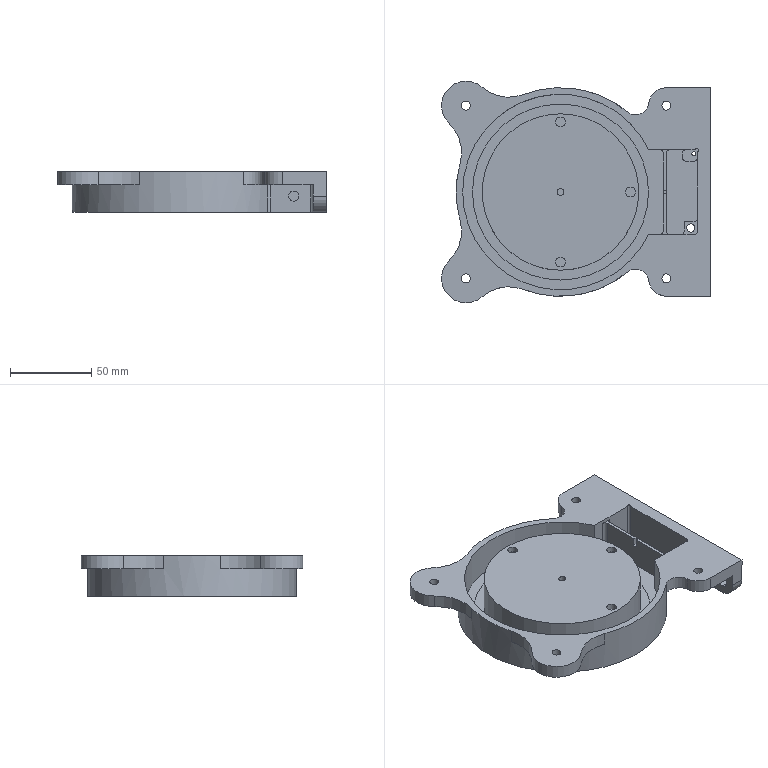NC program | NX | posted with a generic post | part box 165 x 136 x 25 mm
Lines 71 to 1171 of 16615:
(ADAPTIVE_MILLING , TOOL : D10)
N122 T10 M6
N124 G54
N126 G17 G0 G90 X95.139 Y-52.783 S9500 M3
N128 G43 Z30. H10
N130 Z-22.
N132 G94 G1 Z-25. F1000.
N134 X93.885 Y-52.222 F2500.
N136 G3 X92.53 Y-52.783 R1.011
N138 X92.255 Y-53.961 R4.871
N140 X92.058 Y-56.953 R29.061
N142 X92.005 Y-64.578 R349.415
N144 G1 X92.004 Y-66.453
N146 Y-70.016
N148 Y-70.766
N150 Y-70.828
N152 X92.003 Y-70.891
N154 X92.002 Y-70.953
N156 X92. Y-71.015
N158 G2 X90.865 Y-74.007 R5.312
N160 X88.246 Y-76.088 R7.29
N162 X85.091 Y-77.059 R11.809
N164 X81.36 Y-77.407 R28.55
N166 X75.735 Y-77.488 R162.167
N168 G1 X74.923 Y-77.49
N170 X73.985 Y-77.492
N172 X72.673 Y-77.493
N174 X70.798 Y-77.494
N176 X67.36 Y-77.495
N178 X25.735 Y-77.494
N180 X-85.327
N182 X-85.39 Y-77.493
N184 X-85.452 Y-77.492
N186 X-85.515 Y-77.49
N188 G2 X-88.556 Y-76.317 R5.341
N190 X-90.614 Y-73.68 R7.344
N192 X-91.569 Y-70.52 R11.916
N194 X-91.912 Y-66.725 R29.474
N196 X-91.99 Y-60.351 R197.421
N198 G1 X-91.992 Y-59.413
N200 X-91.993 Y-58.101
N202 X-91.994 Y-56.163
N204 X-91.995 Y-52.663
N206 Y6.837
N208 Y70.837
N210 G2 X-90.961 Y73.863 R5.24
N212 X-88.45 Y75.977 R7.1
N214 X-85.317 Y77.014 R11.258
N216 X-81.839 Y77.383 R25.481
N218 X-76.09 Y77.485 R135.933
N220 G1 X-75.34 Y77.488
N222 X-74.465 Y77.489
N224 X-73.403 Y77.491
N226 X-71.903 Y77.492
N228 X-69.528 Y77.493
N230 X-64.09
N232 X-3.653
N234 X-3.403 Y77.494
N236 X85.347
N238 X85.41 Y77.493
N240 X85.472 Y77.492
N242 X85.535 Y77.489
N244 G2 X88.571 Y76.303 R5.343
N246 X90.594 Y73.716 R7.325
N248 X91.56 Y70.559 R11.808
N250 X91.904 Y66.89 R28.115
N252 X91.987 Y61.079 R165.071
N254 G1 X91.989 Y60.266
N256 X91.991 Y59.204
N258 X91.992 Y57.766
N260 X91.993 Y55.641
N262 Y51.266
N264 Y-50.109
N266 X91.992 Y-50.234
N268 X91.991 Y-50.296
N270 X91.99 Y-50.359
N272 G2 X91.814 Y-52.977 R46.721
N274 G3 X91.533 Y-59.97 R91.09
N276 X91.508 Y-68.782 R942.218
N278 G2 X89.291 Y-73.791 R7.073
N280 X86.183 Y-75.732 R9.353
N282 X82.611 Y-76.611 R15.534
N284 X78.374 Y-76.917 R40.348
N286 X70.625 Y-76.987 R304.917
N288 G1 X69.125 Y-76.988
N290 X66.937 Y-76.989
N292 X62.687
N294 X-83.125 Y-76.988
N296 X-83.188
N298 X-83.25
N300 G2 X-88.27 Y-74.797 R7.053
N302 X-90.288 Y-71.521 R9.391
N304 X-91.132 Y-67.94 R16.006
N306 X-91.425 Y-63.514 R44.133
N308 X-91.487 Y-55.952 R338.286
N310 G1 X-91.488 Y-54.452
N312 X-91.489 Y-52.265
N314 Y-47.952
N316 Y-10.577
N318 X-91.491 Y-10.265
N320 Y-9.702
N322 X-91.492 Y-9.39
N324 X-91.491 Y-7.202
N326 X-91.492 Y-6.89
N328 X-91.491 Y-4.702
N330 X-91.492 Y-4.39
N332 X-91.491 Y-2.202
N334 X-91.492 Y-1.89
N336 X-91.491 Y0.298
N338 X-91.492 Y0.61
N340 X-91.491 Y2.798
N342 X-91.492 Y3.11
N344 X-91.491 Y5.298
N346 X-91.492 Y5.61
N348 X-91.491 Y7.798
N350 X-91.492 Y8.11
N352 X-91.491 Y10.298
N354 X-91.492 Y10.61
N356 X-91.491 Y12.798
N358 X-91.492 Y13.11
N360 X-91.491 Y15.298
N362 X-91.492 Y15.61
N364 X-91.491 Y17.798
N366 X-91.492 Y18.11
N368 X-91.491 Y20.298
N370 X-91.492 Y20.61
N372 X-91.491 Y22.798
N374 X-91.492 Y23.11
N376 X-91.491 Y25.298
N378 X-91.492 Y25.61
N380 X-91.491 Y27.798
N382 X-91.492 Y28.11
N384 X-91.491 Y30.298
N386 X-91.492 Y30.61
N388 X-91.491 Y32.798
N390 X-91.492 Y33.11
N392 X-91.491 Y35.298
N394 X-91.492 Y35.61
N396 X-91.491 Y37.798
N398 X-91.492 Y38.11
N400 X-91.491 Y40.298
N402 X-91.492 Y40.61
N404 X-91.491 Y42.798
N406 X-91.492 Y43.11
N408 X-91.491 Y45.298
N410 X-91.492 Y45.61
N412 X-91.491 Y47.798
N414 X-91.492 Y48.11
N416 X-91.491 Y50.298
N418 X-91.492 Y50.61
N420 X-91.491 Y52.798
N422 X-91.492 Y53.11
N424 X-91.491 Y55.298
N426 X-91.492 Y55.61
N428 X-91.491 Y57.798
N430 X-91.492 Y58.11
N432 X-91.491 Y60.298
N434 X-91.492 Y60.61
N436 X-91.491 Y62.798
N438 X-91.492 Y63.11
N440 X-91.491 Y65.298
N442 G2 X-91.484 Y68.985 R228.266
N444 X-89.309 Y73.758 R7.041
N446 X-86.094 Y75.758 R9.386
N448 X-82.455 Y76.628 R15.836
N450 X-78.405 Y76.914 R40.706
N452 X-70.968 Y76.984 R288.617
N454 G1 X-69.655 Y76.986
N456 X-67.843 Y76.987
N458 X-64.843
N460 X-55.405 Y76.988
N462 X-5.843
N464 X-5.718
N466 X-5.093 Y76.989
N468 X83.157
N470 X83.22 Y76.988
N472 X83.282 Y76.987
N474 X83.407 Y76.984
N476 G2 X88.291 Y74.772 R7.043
N478 X90.298 Y71.49 R9.465
N480 X91.136 Y67.907 R16.208
N482 X91.429 Y63.356 R44.995
N484 X91.487 Y54.419 R442.168
N486 G1 Y52.106
N488 X91.488 Y47.356
N490 Y-48.331
N492 X91.486 Y-48.581
N494 X91.485 Y-48.769
N496 X91.483 Y-48.956
N498 G2 X91.288 Y-53.014 R91.927
N500 G3 X91.035 Y-61.509 R150.124
N502 G1 X91.032 Y-62.071
N504 X91.028 Y-62.696
N506 X91.025 Y-63.384
N508 X91.023 Y-64.196
N510 X91.02 Y-65.134
N512 X91.018 Y-66.259
N514 Y-66.446
N516 X91.016 Y-66.696
N518 X91.015 Y-66.821
N520 Y-66.884
N522 X91.012 Y-67.009
N524 X91.011 Y-67.071
N526 G2 X90.235 Y-70.584 R8.586
N528 X87.223 Y-74.019 R8.505
N530 X83.634 Y-75.595 R12.014
N532 X79.629 Y-76.246 R22.581
N534 X74.759 Y-76.445 R71.997
N536 X63.009 Y-76.484 R974.246
N538 G1 X56.322
N540 X-7.491 Y-76.483
N542 X-7.803 Y-76.485
N544 X-8.366
N546 X-8.678 Y-76.486
N548 X-10.866 Y-76.485
N550 X-11.178 Y-76.486
N552 X-13.366 Y-76.485
N554 X-13.678 Y-76.486
N556 X-15.866 Y-76.485
N558 X-16.178 Y-76.486
N560 X-18.366 Y-76.485
N562 X-18.678 Y-76.486
N564 X-20.866 Y-76.485
N566 X-21.178 Y-76.486
N568 X-23.366 Y-76.485
N570 X-23.678 Y-76.486
N572 X-25.866 Y-76.485
N574 X-26.178 Y-76.486
N576 X-28.366 Y-76.485
N578 X-28.678 Y-76.486
N580 X-30.866 Y-76.485
N582 X-31.178 Y-76.486
N584 X-33.366 Y-76.484
N586 X-33.678 Y-76.486
N588 X-35.866 Y-76.484
N590 X-36.178 Y-76.486
N592 X-38.366 Y-76.484
N594 X-38.678 Y-76.486
N596 X-40.866 Y-76.484
N598 X-41.178 Y-76.486
N600 X-43.366 Y-76.484
N602 X-43.678 Y-76.486
N604 X-45.866 Y-76.484
N606 X-46.178 Y-76.486
N608 X-48.366 Y-76.484
N610 X-48.678 Y-76.486
N612 X-50.866 Y-76.484
N614 X-51.178 Y-76.486
N616 X-53.366 Y-76.484
N618 X-53.678 Y-76.486
N620 X-55.866 Y-76.484
N622 X-56.178 Y-76.486
N624 X-58.366 Y-76.484
N626 X-58.678 Y-76.486
N628 X-60.866 Y-76.484
N630 X-61.178 Y-76.486
N632 X-63.366 Y-76.484
N634 X-63.678 Y-76.485
N636 X-65.866 Y-76.484
N638 X-66.178 Y-76.485
N640 X-68.366 Y-76.484
N642 X-68.678 Y-76.485
N644 X-70.866 Y-76.484
N646 X-71.178 Y-76.485
N648 X-73.366 Y-76.484
N650 X-73.678 Y-76.485
N652 X-75.866 Y-76.484
N654 X-76.178 Y-76.485
N656 X-78.366 Y-76.484
N658 G2 X-81.803 Y-76.473 R148.791
N660 X-86.051 Y-75.172 R8.179
N662 X-88.905 Y-72.078 R8.912
N664 X-90.257 Y-68.462 R13.076
N666 X-90.794 Y-64.439 R26.277
N668 X-90.962 Y-58.692 R100.92
N670 X-90.984 Y-49.317 R958.544
N672 G1 Y-44.505
N674 Y-12.755
N676 X-90.985 Y-12.505
N678 X-90.986 Y-11.63
N680 X-90.987 Y-11.317
N682 Y-10.692
N684 X-90.986 Y-9.38
N686 X-90.987 Y-9.13
N688 Y-7.942
N690 Y-7.255
N692 X-90.988 Y-6.942
N694 Y-6.567
N696 X-90.989 Y-6.255
N698 Y-5.942
N700 X-90.99 Y-5.442
N702 X-90.989 Y-4.317
N704 X-90.99 Y-4.005
N706 X-90.989 Y-3.192
N708 X-90.99 Y-2.817
N710 X-90.989 Y-1.755
N712 Y-1.505
N714 X-90.988 Y-0.317
N716 X-90.989 Y-0.005
N718 X-90.988 Y0.745
N720 X-90.989 Y0.933
N722 Y1.558
N724 X-90.99 Y1.87
N726 X-90.988 Y3.183
N728 X-90.989 Y3.433
N730 X-90.988 Y4.62
N732 X-90.989 Y4.933
N734 X-90.988 Y5.808
N736 X-90.989 Y5.995
N738 Y6.558
N740 X-90.988 Y6.745
N742 X-90.989 Y7.058
N744 X-90.988 Y8.245
N746 X-90.989 Y8.495
N748 X-90.988 Y9.683
N750 Y9.87
N752 X-90.989 Y10.183
N754 X-90.988 Y10.808
N756 X-90.989 Y10.933
N758 X-90.988 Y11.62
N760 Y11.745
N762 X-90.989 Y12.058
N764 X-90.988 Y13.245
N766 X-90.989 Y13.495
N768 X-90.988 Y14.683
N770 Y14.808
N772 X-90.989 Y15.12
N774 X-90.988 Y15.808
N776 X-90.989 Y15.995
N778 Y16.62
N780 X-90.99 Y16.933
N782 X-90.988 Y18.183
N784 X-90.989 Y18.433
N786 X-90.988 Y19.558
N788 X-90.989 Y19.87
N790 X-90.988 Y20.745
N792 X-90.989 Y20.933
N794 Y21.37
N796 X-90.988 Y21.745
N798 X-90.989 Y22.058
N800 X-90.988 Y23.245
N802 X-90.989 Y23.433
N804 X-90.988 Y24.058
N806 X-90.989 Y24.37
N808 X-90.988 Y25.745
N810 X-90.989 Y25.995
N812 X-90.988 Y27.183
N814 Y27.308
N816 X-90.989 Y27.62
N818 X-90.988 Y28.308
N820 X-90.989 Y28.433
N822 X-90.988 Y29.058
N824 Y29.433
N826 X-90.989 Y29.745
N828 X-90.988 Y30.808
N830 X-90.989 Y30.995
N832 X-90.988 Y31.558
N834 Y31.745
N836 X-90.989 Y32.058
N838 X-90.988 Y33.245
N840 X-90.989 Y33.433
N842 Y33.87
N844 X-90.988 Y34.12
N846 X-90.989 Y34.433
N848 X-90.988 Y35.745
N850 X-90.989 Y35.933
N852 X-90.988 Y36.558
N854 X-90.989 Y36.87
N856 X-90.988 Y38.245
N858 X-90.989 Y38.433
N860 X-90.988 Y38.87
N862 Y39.12
N864 X-90.989 Y39.433
N866 X-90.988 Y40.745
N868 X-90.989 Y40.933
N870 Y41.37
N872 X-90.988 Y41.745
N874 X-90.989 Y42.058
N876 X-90.988 Y43.245
N878 X-90.989 Y43.433
N880 X-90.988 Y44.058
N882 Y44.12
N884 X-90.989 Y44.433
N886 X-90.988 Y45.683
N888 X-90.989 Y45.933
N890 X-90.988 Y47.058
N892 Y47.308
N894 X-90.989 Y47.62
N896 X-90.988 Y48.308
N898 X-90.989 Y48.433
N900 X-90.988 Y49.12
N902 Y49.37
N904 X-90.989 Y49.683
N906 X-90.988 Y50.745
N908 X-90.99 Y51.245
N910 Y51.37
N912 X-90.991 Y51.87
N914 X-90.989 Y52.87
N916 X-90.991 Y53.683
N918 X-90.989 Y54.745
N920 X-90.99 Y55.12
N922 X-90.989 Y55.745
N924 X-90.99 Y55.995
N926 X-90.989 Y56.933
N928 X-90.99 Y57.308
N930 X-90.989 Y58.245
N932 X-90.99 Y58.495
N934 X-90.988 Y59.62
N936 X-90.99 Y59.995
N938 X-90.989 Y60.808
N940 Y60.995
N942 Y61.433
N944 Y61.808
N946 X-90.99 Y62.183
N948 X-90.989 Y62.433
N950 X-90.99 Y62.808
N952 Y63.245
N954 Y63.433
N956 G2 X-90.979 Y67.245 R266.112
N958 X-89.87 Y71.236 R8.244
N960 X-86.737 Y74.312 R8.787
N962 X-83.14 Y75.714 R12.825
N964 X-79.185 Y76.277 R25.023
N966 X-74.001 Y76.453 R86.031
N968 X-63.251 Y76.482 R987.32
N970 G1 X-57.126
N972 X-26.314
N974 X-26.001 Y76.484
N976 X-25.439 Y76.483
N978 X-25.126 Y76.485
N980 X-22.939 Y76.483
N982 X-22.626 Y76.485
N984 X-20.439 Y76.483
N986 X-20.126 Y76.485
N988 X-17.939 Y76.483
N990 X-17.626 Y76.485
N992 X-15.439 Y76.483
N994 X-15.126 Y76.485
N996 X-12.939 Y76.483
N998 X-12.626 Y76.485
N1000 X-10.439 Y76.483
N1002 X-10.126 Y76.485
N1004 X-8.001 Y76.483
N1006 X-7.814 Y76.484
N1008 X-6.501
N1010 X-6.314
N1012 X-6.001 Y76.485
N1014 X-3.376 Y76.484
N1016 X-3.064 Y76.485
N1018 X-0.314 Y76.484
N1020 X-0.001 Y76.486
N1022 X2.749 Y76.484
N1024 X3.061 Y76.486
N1026 X5.874 Y76.484
N1028 X6.186 Y76.486
N1030 X8.936 Y76.484
N1032 X9.249 Y76.486
N1034 X12.061 Y76.484
N1036 X12.374 Y76.486
N1038 X15.124 Y76.484
N1040 X15.436 Y76.486
N1042 X18.249 Y76.484
N1044 X18.561 Y76.486
N1046 X21.311 Y76.484
N1048 X21.624 Y76.486
N1050 X24.436 Y76.484
N1052 X24.749 Y76.486
N1054 X27.499 Y76.484
N1056 X27.811 Y76.486
N1058 X30.624 Y76.484
N1060 X30.936 Y76.486
N1062 X33.749 Y76.484
N1064 X34.061 Y76.486
N1066 X36.811 Y76.484
N1068 X37.124 Y76.486
N1070 X39.936 Y76.484
N1072 X40.249 Y76.486
N1074 X42.999 Y76.484
N1076 X43.311 Y76.486
N1078 X46.124 Y76.484
N1080 X46.436 Y76.486
N1082 X49.186 Y76.484
N1084 X49.499 Y76.486
N1086 X52.311 Y76.484
N1088 X52.624 Y76.486
N1090 X55.374 Y76.484
N1092 X55.686 Y76.486
N1094 X58.499 Y76.484
N1096 X58.811 Y76.486
N1098 X61.561 Y76.484
N1100 X61.874 Y76.486
N1102 X64.686 Y76.484
N1104 X64.999 Y76.486
N1106 X67.749 Y76.484
N1108 X68.061 Y76.486
N1110 X70.874 Y76.484
N1112 X71.186 Y76.486
N1114 X73.936 Y76.484
N1116 X74.249 Y76.486
N1118 X77.061 Y76.484
N1120 X77.374 Y76.486
N1122 X80.124 Y76.484
N1124 X80.436 Y76.486
N1126 X81.186 Y76.485
N1128 X81.374 Y76.484
N1130 X81.436
N1132 X81.561 Y76.481
N1134 G2 X85.076 Y75.714 R8.483
N1136 X88.617 Y72.55 R8.518
N1138 X90.125 Y68.999 R12.224
N1140 X90.756 Y64.991 R23.353
N1142 X90.95 Y59.808 R79.617
N1144 X90.982 Y50.433 R858.768
N1146 G1 Y46.933
N1148 X90.983 Y30.495
N1150 X90.982 Y-47.005
N1152 X90.981 Y-47.255
N1154 X90.978 Y-47.567
N1156 G2 X90.795 Y-52.626 R117.036
N1158 G3 X90.538 Y-62.934 R211.978
N1160 G2 X90.5 Y-65.996 R87.112
N1162 X89.684 Y-69.569 R9.654
N1164 X86.365 Y-73.385 R9.11
N1166 X82.662 Y-75.014 R12.786
N1168 X78.6 Y-75.701 R23.382
N1170 X73.481 Y-75.932 R70.527
N1172 X62.356 Y-75.978 R790.426
N1174 G1 X58.356
N1176 X21.731
N1178 X-5.331
N1180 X-5.644 Y-75.98
N1182 X-6.206
N1184 X-6.581 Y-75.981
N1186 X-7.581
N1188 X-8.269
N1190 X-8.581 Y-75.982
N1192 X-9.019
N1194 X-9.331 Y-75.983
N1196 X-9.769 Y-75.982
N1198 X-10.206 Y-75.984
N1200 X-10.456 Y-75.983
N1202 X-10.831 Y-75.984
N1204 X-11.393 Y-75.983
N1206 X-11.581 Y-75.984
N1208 X-12.831 Y-75.983
N1210 X-13.206 Y-75.984
N1212 X-13.893 Y-75.983
N1214 X-14.081
N1216 X-14.706
N1218 X-14.831
N1220 X-15.518
N1222 X-15.893 Y-75.984
N1224 X-16.393 Y-75.983
N1226 X-16.581 Y-75.984
N1228 X-17.206 Y-75.983
N1230 X-17.331
N1232 X-18.831 Y-75.982
N1234 X-19.018 Y-75.983
N1236 X-19.581 Y-75.982
N1238 X-19.768
N1240 X-19.893 Y-75.983
N1242 X-20.893 Y-75.982
N1244 X-21.143
N1246 X-21.518 Y-75.983
N1248 X-22.331 Y-75.982
N1250 X-22.706 Y-75.984
N1252 X-23.018 Y-75.983
N1254 X-23.643 Y-75.985
N1256 X-23.956 Y-75.984
N1258 X-24.581 Y-75.986
N1260 X-24.706 Y-75.985
N1262 X-25.456 Y-75.987
N1264 X-26.081 Y-75.985
N1266 X-26.643 Y-75.986
N1268 X-26.768
N1270 X-27.456 Y-75.987
N1272 X-28.081 Y-75.985
N1274 X-29.268 Y-75.987
N1276 X-29.893 Y-75.986
N1278 X-30.518 Y-75.987
N1280 X-31.143 Y-75.985
N1282 X-31.643 Y-75.986
N1284 X-31.768
N1286 X-32.456 Y-75.987
N1288 X-33.081 Y-75.985
N1290 X-34.268 Y-75.987
N1292 X-34.893 Y-75.986
N1294 X-35.518 Y-75.987
N1296 X-36.143 Y-75.985
N1298 X-36.706 Y-75.986
N1300 X-36.831
N1302 X-37.706 Y-75.987
N1304 X-37.831
N1306 X-39.268 Y-75.988
N1308 X-39.768 Y-75.987
N1310 X-40.456
N1312 X-40.956 Y-75.986
N1314 X-41.581 Y-75.987
N1316 X-41.706 Y-75.986
N1318 X-43.018 Y-75.988
N1320 X-44.331 Y-75.989
N1322 X-45.643
N1324 X-46.956 Y-75.988
N1326 X-48.268 Y-75.986
N1328 X-49.518 Y-75.984
N1330 X-50.018 Y-75.985
N1332 X-50.143
N1334 X-50.956 Y-75.986
N1336 X-51.081
N1338 X-51.768 Y-75.987
N1340 X-51.893
N1342 X-52.018
N1344 X-53.331 Y-75.988
N1346 X-54.643 Y-75.989
N1348 X-55.956 Y-75.988
N1350 X-57.268
N1352 X-58.581 Y-75.986
N1354 X-59.706 Y-75.984
N1356 X-60.143 Y-75.985
N1358 X-61.018 Y-75.983
N1360 X-61.956 Y-75.986
N1362 X-62.081 Y-75.985
N1364 X-62.893 Y-75.987
N1366 X-63.018 Y-75.986
N1368 X-64.581 Y-75.988
N1370 X-65.081 Y-75.986
N1372 X-65.768 Y-75.987
N1374 X-66.206 Y-75.986
N1376 X-66.768 Y-75.987
N1378 X-66.893 Y-75.986
N1380 X-67.768 Y-75.987
N1382 X-67.893
N1384 X-69.331 Y-75.988
N1386 X-69.456
N1388 X-69.956 Y-75.987
N1390 X-70.768
N1392 X-71.206 Y-75.986
N1394 X-71.831 Y-75.987
N1396 X-72.456 Y-75.985
N1398 X-73.081 Y-75.986
N1400 X-73.706 Y-75.985
N1402 X-74.268 Y-75.986
N1404 G2 X-80.143 Y-75.976 R612.966
N1406 X-83.277 Y-75.467 R10.413
N1408 X-87.615 Y-72.23 R8.912
N1410 X-89.383 Y-68.593 R12.154
N1412 X-90.147 Y-64.609 R21.448
N1414 X-90.418 Y-59.681 R58.799
N1416 X-90.477 Y-49.744 R542.864
N1418 G1 X-90.478 Y-47.369
N1420 X-90.479 Y-42.806
N1422 Y-14.931
N1424 X-90.48 Y-14.619
N1426 Y-13.744
N1428 X-90.482 Y-13.494
N1430 Y-12.431
N1432 Y-11.556
N1434 X-90.483 Y-11.244
N1436 Y-10.181
N1438 Y-9.431
N1440 X-90.484 Y-9.181
N1442 Y-8.494
N1444 Y-8.369
N1446 X-90.485 Y-7.806
N1448 Y-7.619
N1450 Y-6.994
N1452 Y-6.494
N1454 X-90.486 Y-6.181
N1456 Y-5.244
N1458 Y-5.056
N1460 Y-4.619
N1462 Y-3.931
N1464 X-90.487 Y-3.681
N1466 X-90.486 Y-2.556
N1468 Y-2.431
N1470 Y-2.181
N1472 Y-1.244
N1474 X-90.487 Y-0.869
N1476 Y-0.619
N1478 X-90.488 Y0.006
N1480 Y0.444
N1482 X-90.489 Y0.881
N1484 X-90.488 Y1.256
N1486 X-90.489 Y1.756
N1488 X-90.487 Y2.569
N1490 X-90.488 Y2.881
N1492 X-90.487 Y3.694
N1494 X-90.488 Y3.944
N1496 X-90.487 Y4.694
N1498 Y4.944
N1500 X-90.486 Y6.006
N1502 X-90.487 Y6.319
N1504 X-90.486 Y7.069
N1506 X-90.487 Y7.381
N1508 X-90.486 Y7.944
N1510 X-90.487 Y8.069
N1512 X-90.486 Y8.756
N1514 X-90.487 Y8.881
N1516 X-90.486 Y9.756
N1518 Y9.881
N1520 Y10.569
N1522 X-90.485 Y11.069
N1524 X-90.486 Y11.381
N1526 X-90.485 Y12.381
N1528 X-90.487 Y13.006
N1530 Y13.194
N1532 X-90.489 Y14.256
N1534 X-90.491 Y15.381
N1536 X-90.492 Y16.506
N1538 Y17.631
N1540 X-90.491 Y18.756
N1542 X-90.49 Y19.881
N1544 X-90.488 Y20.819
N1546 X-90.489 Y21.569
N1548 X-90.488 Y22.006
N1550 X-90.489 Y22.256
N1552 X-90.487 Y23.194
N1554 X-90.489 Y23.944
N1556 X-90.487 Y24.819
N1558 X-90.489 Y25.631
N1560 Y25.756
N1562 X-90.49 Y26.694
N1564 X-90.489 Y27.319
N1566 X-90.49 Y27.756
N1568 X-90.489 Y28.131
N1570 X-90.49 Y29.194
N1572 X-90.489 Y29.694
N1574 X-90.49 Y30.006
N1576 X-90.488 Y30.631
N1578 X-90.49 Y31.381
N1580 X-90.488 Y32.006
N1582 X-90.489 Y32.381
N1584 X-90.488 Y33.006
N1586 X-90.489 Y33.381
N1588 X-90.488 Y33.756
N1590 X-90.489 Y34.319
N1592 X-90.488 Y34.631
N1594 X-90.49 Y35.131
N1596 X-90.487 Y36.131
N1598 X-90.488 Y36.381
N1600 X-90.487 Y37.006
N1602 X-90.488 Y37.319
N1604 X-90.487 Y38.194
N1606 X-90.488 Y38.569
N1608 X-90.487 Y39.006
N1610 X-90.488 Y39.381
N1612 X-90.487 Y39.756
N1614 X-90.489 Y40.256
N1616 X-90.488 Y40.444
N1618 X-90.489 Y40.881
N1620 X-90.488 Y41.256
N1622 X-90.489 Y41.756
N1624 X-90.488 Y42.131
N1626 X-90.49 Y42.694
N1628 X-90.488 Y43.569
N1630 Y43.881
N1632 X-90.487 Y44.569
N1634 X-90.488 Y44.944
N1636 X-90.487 Y45.319
N1638 X-90.489 Y45.819
N1640 X-90.487 Y46.444
N1642 X-90.488 Y46.881
N1644 Y47.381
N1646 Y47.569
N1648 X-90.487 Y48.131
N1650 X-90.488 Y48.506
N1652 Y48.819
N1654 X-90.489 Y49.194
N1656 X-90.488 Y49.631
N1658 X-90.489 Y49.944
N1660 X-90.488 Y50.694
N1662 X-90.489 Y51.194
N1664 X-90.487 Y52.694
N1666 X-90.488 Y52.881
N1668 X-90.487 Y53.506
N1670 Y53.569
N1672 X-90.488 Y53.881
N1674 X-90.487 Y54.756
N1676 X-90.488 Y55.131
N1678 X-90.487 Y56.069
N1680 X-90.488 Y56.381
N1682 X-90.487 Y57.319
N1684 X-90.489 Y58.069
N1686 X-90.488 Y58.319
N1688 X-90.49 Y58.944
N1690 X-90.489 Y59.069
N1692 X-90.49 Y59.569
N1694 X-90.489 Y59.881
N1696 X-90.491 Y60.819
N1698 Y60.944
N1700 X-90.492 Y61.881
N1702 X-90.49 Y62.444
N1704 G2 X-90.475 Y65.818 R135.493
N1706 X-89.824 Y69.176 R9.958
N1708 X-86.589 Y73.216 R8.972
N1710 X-82.927 Y74.932 R12.352
N1712 X-78.937 Y75.666 R22.255
N1714 X-73.82 Y75.924 R63.881
N1716 X-64.257 Y75.975 R594.582
N1718 G1 X-61.82 Y75.976
N1720 X-57.195 Y75.977
N1722 X-28.507
N1724 X-28.382
N1726 X-27.757 Y75.978
N1728 X-27.632
N1730 X-27.445 Y75.979
N1732 X-26.507
N1734 X-25.132
N1736 X-25.007
N1738 X-24.507 Y75.98
N1740 X-22.632 Y75.979
N1742 X-22.507
N1744 X-22.007 Y75.98
N1746 X-20.132 Y75.979
N1748 X-20.007 Y75.98
N1750 X-19.507
N1752 X-17.632 Y75.979
N1754 X-17.507 Y75.98
N1756 X-17.007
N1758 X-15.132 Y75.979
N1760 X-15.007 Y75.98
N1762 X-14.507
N1764 X-12.507 Y75.979
N1766 X-12.32 Y75.98
N1768 X-11.695
N1770 X-10.445 Y75.979
N1772 X-9.945 Y75.981
N1774 X-8.382 Y75.98
N1776 X-8.195 Y75.981
N1778 X-7.632
N1780 X-6.882
N1782 X-6.57 Y75.982
N1784 X-6.257
N1786 X-5.757 Y75.983
N1788 X-5.382
N1790 X-4.882 Y75.984
N1792 X-3.632 Y75.982
N1794 X-3.257 Y75.984
N1796 X-2.382 Y75.982
N1798 X-2.132 Y75.983
N1800 X-1.132 Y75.982
N1802 X-0.82 Y75.983
N1804 X0.555 Y75.982
N1806 X0.868 Y75.983
N1808 X1.68 Y75.982
N1810 X1.993 Y75.983
N1812 X3.618 Y75.981
N1814 X4.305 Y75.984
N1816 X6.055 Y75.982
N1818 X6.368 Y75.983
N1820 X6.93 Y75.982
N1822 X7.118 Y75.983
N1824 X7.743 Y75.982
N1826 X8.118 Y75.984
N1828 X9.868 Y75.982
N1830 X10.18 Y75.983
N1832 X10.993 Y75.982
N1834 X11.305 Y75.983
N1836 X12.93 Y75.981
N1838 X13.243 Y75.982
N1840 X14.18
N1842 X14.493 Y75.983
N1844 X16.118 Y75.981
N1846 X16.368 Y75.982
N1848 X17.493
N1850 X17.743 Y75.981
N1852 X18.055 Y75.983
N1854 X19.305 Y75.981
N1856 X19.493 Y75.982
N1858 X20.055
N1860 X20.305
N1862 X20.618 Y75.983
N1864 X22.368 Y75.981
N1866 X22.618 Y75.982
N1868 X23.805
N1870 X24.055 Y75.981
N1872 X24.368 Y75.982
N1874 X25.493
N1876 X25.68
N1878 X26.243
N1880 X26.618
N1882 X26.93 Y75.983
N1884 X28.555 Y75.981
N1886 X28.805 Y75.982
N1888 X29.993
N1890 X30.18 Y75.981
N1892 X30.493 Y75.983
N1894 X31.68 Y75.981
N1896 X32.18 Y75.983
N1898 X34.618 Y75.981
N1900 X34.93 Y75.982
N1902 X35.93
N1904 X36.243 Y75.983
N1906 X37.868 Y75.981
N1908 X38.118 Y75.982
N1910 X39.305
N1912 X39.493
N1914 X39.805 Y75.983
N1916 X40.93 Y75.982
N1918 X41.118
N1920 X41.68
N1922 X41.868
N1924 X42.18 Y75.983
N1926 X43.993 Y75.981
N1928 X44.18 Y75.982
N1930 X44.743
N1932 X45.055 Y75.983
N1934 X46.993 Y75.981
N1936 X47.305 Y75.982
N1938 X48.305
N1940 X48.618 Y75.983
N1942 X50.243 Y75.981
N1944 X50.43 Y75.982
N1946 X50.868
N1948 X51.243
N1950 X51.555 Y75.983
N1952 X53.305 Y75.981
N1954 X53.493 Y75.982
N1956 X53.93
N1958 X54.243
N1960 X54.555 Y75.983
N1962 X56.43 Y75.981
N1964 X56.618 Y75.982
N1966 X57.055
N1968 X57.43
N1970 X57.743 Y75.983
N1972 X59.493 Y75.981
N1974 X59.618 Y75.982
N1976 X60.243
N1978 X60.493 Y75.981
N1980 X60.805 Y75.983
N1982 X62.68 Y75.981
N1984 X62.868 Y75.982
N1986 X63.43
N1988 X63.93 Y75.981
N1990 X64.243 Y75.983
N1992 X65.743 Y75.981
N1994 X65.93 Y75.982
N1996 X66.493
N1998 X66.93
N2000 X67.243 Y75.983
N2002 X68.805 Y75.981
N2004 X68.993 Y75.982
N2006 X69.618
N2008 X69.93 Y75.983
N2010 X71.805 Y75.981
N2012 X72.117 Y75.982
N2014 X73.242
N2016 X73.555 Y75.983
N2018 X74.992 Y75.981
N2020 X75.18 Y75.982
N2022 X75.742
N2024 X76.055 Y75.983
N2026 X77.617 Y75.981
N2028 G2 X80.555 Y75.959 R68.776
N2030 X84.237 Y75.075 R9.482
N2032 X87.92 Y71.786 R9.144
N2034 X89.531 Y68.075 R12.828
N2036 X90.218 Y63.887 R23.879
N2038 X90.44 Y58.393 R80.072
N2040 X90.476 Y48.518 R864.782
N2042 G1 X90.477 Y45.205
N2044 Y34.83
N2046 Y-45.982
N2048 X90.476 Y-46.17
N2050 X90.474 Y-46.42
N2052 G2 X90.291 Y-52.479 R153.217
N2054 G3 X90.045 Y-63.038 R269.347
N2056 G2 X89.943 Y-65.535 R26.924
N2058 X88.544 Y-69.77 R9.815
N2060 X85.046 Y-73.097 R10.027
N2062 X81.156 Y-74.604 R14.293
N2064 X76.706 Y-75.242 R27.866
N2066 X70.836 Y-75.441 R96.727
N2068 X60.898 Y-75.472 R914.91
N2070 G1 X57.398 Y-75.473
N2072 X45.648
N2074 X-3.102
N2076 X-3.789 Y-75.476
N2078 X-3.914
N2080 X-4.477 Y-75.478
N2082 X-4.727
N2084 X-4.977 Y-75.479
N2086 X-5.352 Y-75.478
N2088 X-5.727 Y-75.479
N2090 X-6.164
N2092 X-6.414 Y-75.48
N2094 X-6.977 Y-75.479
N2096 X-7.414 Y-75.481
N2098 X-7.602 Y-75.48
N2100 X-8.102 Y-75.482
N2102 X-8.289
N2104 X-8.789 Y-75.483
N2106 X-10.102 Y-75.481
N2108 X-10.414 Y-75.482
N2110 X-10.914 Y-75.481
N2112 X-11.289 Y-75.482
N2114 X-12.227 Y-75.481
N2116 X-12.664 Y-75.482
N2118 X-13.539 Y-75.481
N2120 X-13.977 Y-75.482
N2122 X-14.727 Y-75.481
N2124 X-15.164 Y-75.483
N2126 X-16.789 Y-75.48
N2128 X-17.227 Y-75.481
N2130 X-18.039 Y-75.48
N2132 X-18.352 Y-75.481
N2134 X-19.102 Y-75.48
N2136 X-19.352 Y-75.481
N2138 X-20.289 Y-75.48
N2140 X-20.539 Y-75.481
N2142 X-21.164 Y-75.48
N2144 X-21.289 Y-75.481
N2146 X-22.164
N2148 X-22.539 Y-75.482
N2150 X-23.102
N2152 X-23.352 Y-75.483
N2154 X-23.977 Y-75.482
N2156 X-24.102
N2158 X-24.289 Y-75.483
N2160 X-24.852
N2162 X-25.289 Y-75.484
N2164 X-25.977 Y-75.483
N2166 X-26.914 Y-75.486
N2168 X-28.102 Y-75.484
N2170 X-28.477 Y-75.485
N2172 X-29.039 Y-75.484
N2174 X-29.227 Y-75.485
N2176 X-29.664 Y-75.484
N2178 X-30.352 Y-75.486
N2180 X-30.977 Y-75.485
N2182 X-32.227 Y-75.487
N2184 X-32.789 Y-75.486
N2186 X-33.352 Y-75.487
N2188 X-33.977 Y-75.486
N2190 X-34.602 Y-75.487
N2192 X-34.789 Y-75.486
N2194 X-35.227 Y-75.487
N2196 X-35.477 Y-75.488
N2198 X-35.727 Y-75.487
N2200 X-36.539 Y-75.489
N2202 X-36.977 Y-75.488
N2204 X-37.164
N2206 X-37.789 Y-75.487
N2208 X-37.852
N2210 X-38.227 Y-75.488
N2212 X-38.977 Y-75.486
N2214 X-39.227
N2216 X-39.664
N2218 X-40.789 Y-75.488
N2220 X-41.227 Y-75.487
N2222 X-41.914 Y-75.489
N2224 X-42.477 Y-75.488
N2226 X-43.039 Y-75.489
N2228 X-43.164
N2230 X-44.102 Y-75.49
N2232 X-44.227
N2234 X-45.227 Y-75.491
N2236 X-45.352 Y-75.49
N2238 X-46.352 Y-75.491
N2240 X-46.477 Y-75.49
N2242 X-47.977
N2244 X-49.352
N2246 X-49.789 Y-75.491
N2248 X-49.914 Y-75.49
N2250 X-50.539
N2252 X-51.102 Y-75.491
N2254 X-51.477 Y-75.49
N2256 X-51.852
N2258 X-52.102 Y-75.489
N2260 X-52.539 Y-75.49
N2262 X-53.102 Y-75.489
N2264 X-53.227
N2266 X-54.289 Y-75.487
N2268 X-54.727 Y-75.488
N2270 X-54.977
N2272 X-55.414
N2274 X-55.664
N2276 X-56.414 Y-75.489
N2278 X-56.539 Y-75.488
N2280 X-57.477 Y-75.489
N2282 X-57.602 Y-75.488
N2284 X-58.289
N2286 X-58.477
N2288 X-58.727 Y-75.487
N2290 X-59.602 Y-75.488
N2292 X-60.727 Y-75.489
N2294 X-60.914 Y-75.488
N2296 X-61.539 Y-75.489
N2298 X-61.602
N2300 X-61.727
N2302 X-62.414 Y-75.49
N2304 X-62.977 Y-75.488
N2306 X-63.477 Y-75.489
N2308 X-63.602 Y-75.488
N2310 X-64.477 Y-75.489
N2312 X-65.414
N2314 X-66.352 Y-75.488
N2316 X-67.289 Y-75.487